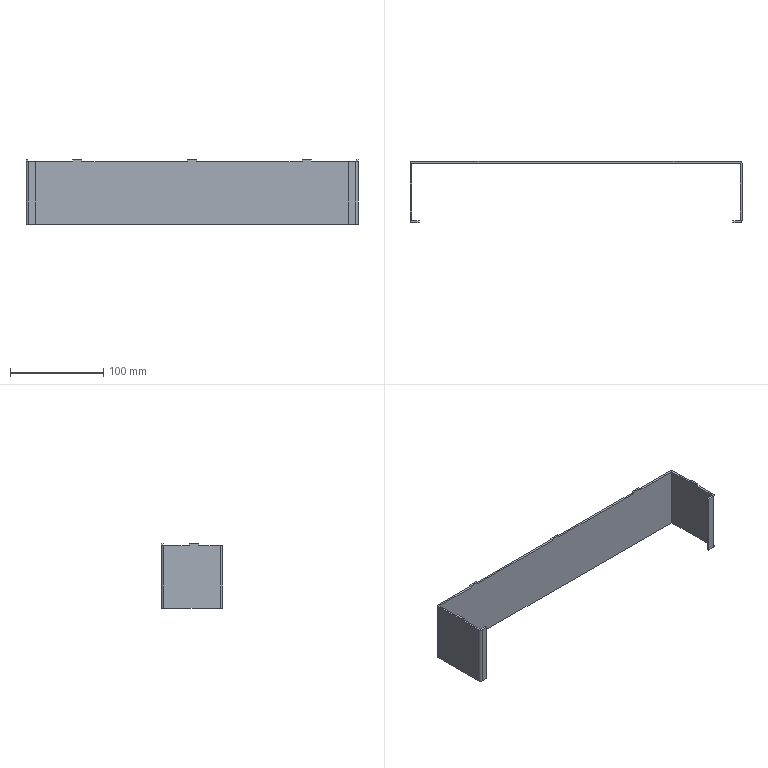Part | STEP file | xzz-005 | 1 solid | 42 faces | box 356 x 66 x 69 mm | volume 66855 mm3 | plane 34 | cylinder 8 | commonest cylinder face diameters 1 x4 5 x4
STEP:
#1=CARTESIAN_POINT('',(198.5,6.,67.));
#2=VERTEX_POINT('',#1);
#3=CARTESIAN_POINT('',(198.5,6.,0.));
#4=VERTEX_POINT('',#3);
#5=CARTESIAN_POINT('',(198.5,6.,67.));
#6=DIRECTION('',(0.,0.,-1.));
#7=VECTOR('',#6,1000.);
#8=LINE('',#5,#7);
#9=EDGE_CURVE('',#2,#4,#8,.T.);
#10=ORIENTED_EDGE('',*,*,#9,.F.);
#11=CARTESIAN_POINT('',(151.,6.,67.));
#12=VERTEX_POINT('',#11);
#13=CARTESIAN_POINT('',(-155.,6.,67.));
#14=DIRECTION('',(1.,0.,0.));
#15=VECTOR('',#14,1000.);
#16=LINE('',#13,#15);
#17=EDGE_CURVE('',#12,#2,#16,.T.);
#18=ORIENTED_EDGE('',*,*,#17,.F.);
#19=CARTESIAN_POINT('',(151.,6.,69.));
#20=VERTEX_POINT('',#19);
#21=CARTESIAN_POINT('',(151.,6.,67.));
#22=DIRECTION('',(0.,0.,-1.));
#23=VECTOR('',#22,1000.);
#24=LINE('',#21,#23);
#25=EDGE_CURVE('',#20,#12,#24,.T.);
#26=ORIENTED_EDGE('',*,*,#25,.F.);
#27=CARTESIAN_POINT('',(141.,6.,69.));
#28=VERTEX_POINT('',#27);
#29=CARTESIAN_POINT('',(-155.,6.,69.));
#30=DIRECTION('',(1.,0.,0.));
#31=VECTOR('',#30,1000.);
#32=LINE('',#29,#31);
#33=EDGE_CURVE('',#28,#20,#32,.T.);
#34=ORIENTED_EDGE('',*,*,#33,.F.);
#35=CARTESIAN_POINT('',(141.,6.,67.));
#36=VERTEX_POINT('',#35);
#37=CARTESIAN_POINT('',(141.,6.,67.));
#38=DIRECTION('',(0.,0.,1.));
#39=VECTOR('',#38,1000.);
#40=LINE('',#37,#39);
#41=EDGE_CURVE('',#36,#28,#40,.T.);
#42=ORIENTED_EDGE('',*,*,#41,.F.);
#43=CARTESIAN_POINT('',(28.,6.,67.));
#44=VERTEX_POINT('',#43);
#45=CARTESIAN_POINT('',(-155.,6.,67.));
#46=DIRECTION('',(1.,0.,0.));
#47=VECTOR('',#46,1000.);
#48=LINE('',#45,#47);
#49=EDGE_CURVE('',#44,#36,#48,.T.);
#50=ORIENTED_EDGE('',*,*,#49,.F.);
#51=CARTESIAN_POINT('',(28.,6.,69.));
#52=VERTEX_POINT('',#51);
#53=CARTESIAN_POINT('',(28.,6.,67.));
#54=DIRECTION('',(0.,0.,-1.));
#55=VECTOR('',#54,1000.);
#56=LINE('',#53,#55);
#57=EDGE_CURVE('',#52,#44,#56,.T.);
#58=ORIENTED_EDGE('',*,*,#57,.F.);
#59=CARTESIAN_POINT('',(18.,6.,69.));
#60=VERTEX_POINT('',#59);
#61=CARTESIAN_POINT('',(-155.,6.,69.));
#62=DIRECTION('',(1.,0.,0.));
#63=VECTOR('',#62,1000.);
#64=LINE('',#61,#63);
#65=EDGE_CURVE('',#60,#52,#64,.T.);
#66=ORIENTED_EDGE('',*,*,#65,.F.);
#67=CARTESIAN_POINT('',(18.,6.,67.));
#68=VERTEX_POINT('',#67);
#69=CARTESIAN_POINT('',(18.,6.,67.));
#70=DIRECTION('',(0.,0.,1.));
#71=VECTOR('',#70,1000.);
#72=LINE('',#69,#71);
#73=EDGE_CURVE('',#68,#60,#72,.T.);
#74=ORIENTED_EDGE('',*,*,#73,.F.);
#75=CARTESIAN_POINT('',(-95.,6.,67.));
#76=VERTEX_POINT('',#75);
#77=CARTESIAN_POINT('',(-155.,6.,67.));
#78=DIRECTION('',(1.,0.,0.));
#79=VECTOR('',#78,1000.);
#80=LINE('',#77,#79);
#81=EDGE_CURVE('',#76,#68,#80,.T.);
#82=ORIENTED_EDGE('',*,*,#81,.F.);
#83=CARTESIAN_POINT('',(-95.,6.,69.));
#84=VERTEX_POINT('',#83);
#85=CARTESIAN_POINT('',(-95.,6.,67.));
#86=DIRECTION('',(0.,0.,-1.));
#87=VECTOR('',#86,1000.);
#88=LINE('',#85,#87);
#89=EDGE_CURVE('',#84,#76,#88,.T.);
#90=ORIENTED_EDGE('',*,*,#89,.F.);
#91=CARTESIAN_POINT('',(-105.,6.,69.));
#92=VERTEX_POINT('',#91);
#93=CARTESIAN_POINT('',(-155.,6.,69.));
#94=DIRECTION('',(1.,0.,0.));
#95=VECTOR('',#94,1000.);
#96=LINE('',#93,#95);
#97=EDGE_CURVE('',#92,#84,#96,.T.);
#98=ORIENTED_EDGE('',*,*,#97,.F.);
#99=CARTESIAN_POINT('',(-105.,6.,67.));
#100=VERTEX_POINT('',#99);
#101=CARTESIAN_POINT('',(-105.,6.,67.));
#102=DIRECTION('',(0.,0.,1.));
#103=VECTOR('',#102,1000.);
#104=LINE('',#101,#103);
#105=EDGE_CURVE('',#100,#92,#104,.T.);
#106=ORIENTED_EDGE('',*,*,#105,.F.);
#107=CARTESIAN_POINT('',(-152.5,6.,67.));
#108=VERTEX_POINT('',#107);
#109=CARTESIAN_POINT('',(-155.,6.,67.));
#110=DIRECTION('',(1.,0.,0.));
#111=VECTOR('',#110,1000.);
#112=LINE('',#109,#111);
#113=EDGE_CURVE('',#108,#100,#112,.T.);
#114=ORIENTED_EDGE('',*,*,#113,.F.);
#115=CARTESIAN_POINT('',(-152.5,6.,0.));
#116=VERTEX_POINT('',#115);
#117=CARTESIAN_POINT('',(-152.5,6.,67.));
#118=DIRECTION('',(0.,0.,1.));
#119=VECTOR('',#118,1000.);
#120=LINE('',#117,#119);
#121=EDGE_CURVE('',#116,#108,#120,.T.);
#122=ORIENTED_EDGE('',*,*,#121,.F.);
#123=CARTESIAN_POINT('',(-155.,6.,0.));
#124=DIRECTION('',(-1.,0.,0.));
#125=VECTOR('',#124,1000.);
#126=LINE('',#123,#125);
#127=EDGE_CURVE('',#4,#116,#126,.T.);
#128=ORIENTED_EDGE('',*,*,#127,.F.);
#129=EDGE_LOOP('',(#10,#18,#26,#34,#42,#50,#58,#66,#74,#82,#90,#98,#106,#114,#122,#128));
#130=FACE_OUTER_BOUND('',#129,.T.);
#131=CARTESIAN_POINT('',(-155.,6.,67.));
#132=DIRECTION('',(0.,1.,0.));
#133=DIRECTION('',(0.,0.,1.));
#134=AXIS2_PLACEMENT_3D('',#131,#132,#133);
#135=PLANE('',#134);
#136=ADVANCED_FACE('',(#130),#135,.F.);
#137=ORIENTED_EDGE('',*,*,#127,.T.);
#138=CARTESIAN_POINT('',(-153.,5.5,0.));
#139=VERTEX_POINT('',#138);
#140=CARTESIAN_POINT('',(-152.5,5.5,0.));
#141=DIRECTION('',(0.,0.,1.));
#142=DIRECTION('',(-1.,0.,0.));
#143=AXIS2_PLACEMENT_3D('',#140,#141,#142);
#144=CIRCLE('',#143,0.5);
#145=EDGE_CURVE('',#116,#139,#144,.T.);
#146=ORIENTED_EDGE('',*,*,#145,.T.);
#147=CARTESIAN_POINT('',(-153.,-55.5,0.));
#148=VERTEX_POINT('',#147);
#149=CARTESIAN_POINT('',(-153.,8.,0.));
#150=DIRECTION('',(0.,-1.,0.));
#151=VECTOR('',#150,1000.);
#152=LINE('',#149,#151);
#153=EDGE_CURVE('',#139,#148,#152,.T.);
#154=ORIENTED_EDGE('',*,*,#153,.T.);
#155=CARTESIAN_POINT('',(-152.5,-56.,0.));
#156=VERTEX_POINT('',#155);
#157=CARTESIAN_POINT('',(-152.5,-55.5,0.));
#158=DIRECTION('',(0.,0.,1.));
#159=DIRECTION('',(-1.,0.,0.));
#160=AXIS2_PLACEMENT_3D('',#157,#158,#159);
#161=CIRCLE('',#160,0.5);
#162=EDGE_CURVE('',#148,#156,#161,.T.);
#163=ORIENTED_EDGE('',*,*,#162,.T.);
#164=CARTESIAN_POINT('',(-145.,-56.,0.));
#165=VERTEX_POINT('',#164);
#166=CARTESIAN_POINT('',(-155.,-56.,0.));
#167=DIRECTION('',(1.,0.,0.));
#168=VECTOR('',#167,1000.);
#169=LINE('',#166,#168);
#170=EDGE_CURVE('',#156,#165,#169,.T.);
#171=ORIENTED_EDGE('',*,*,#170,.T.);
#172=CARTESIAN_POINT('',(-145.,-58.,0.));
#173=VERTEX_POINT('',#172);
#174=CARTESIAN_POINT('',(-145.,-55.5,0.));
#175=DIRECTION('',(0.,-1.,0.));
#176=VECTOR('',#175,1000.);
#177=LINE('',#174,#176);
#178=EDGE_CURVE('',#165,#173,#177,.T.);
#179=ORIENTED_EDGE('',*,*,#178,.T.);
#180=CARTESIAN_POINT('',(-152.5,-58.,0.));
#181=VERTEX_POINT('',#180);
#182=CARTESIAN_POINT('',(-153.,-58.,0.));
#183=DIRECTION('',(-1.,0.,0.));
#184=VECTOR('',#183,1000.);
#185=LINE('',#182,#184);
#186=EDGE_CURVE('',#173,#181,#185,.T.);
#187=ORIENTED_EDGE('',*,*,#186,.T.);
#188=CARTESIAN_POINT('',(-155.,-55.5,0.));
#189=VERTEX_POINT('',#188);
#190=CARTESIAN_POINT('',(-152.5,-55.5,0.));
#191=DIRECTION('',(0.,0.,-1.));
#192=DIRECTION('',(-1.,0.,0.));
#193=AXIS2_PLACEMENT_3D('',#190,#191,#192);
#194=CIRCLE('',#193,2.5);
#195=EDGE_CURVE('',#181,#189,#194,.T.);
#196=ORIENTED_EDGE('',*,*,#195,.T.);
#197=CARTESIAN_POINT('',(-155.,5.5,0.));
#198=VERTEX_POINT('',#197);
#199=CARTESIAN_POINT('',(-155.,6.,0.));
#200=DIRECTION('',(0.,1.,0.));
#201=VECTOR('',#200,1000.);
#202=LINE('',#199,#201);
#203=EDGE_CURVE('',#189,#198,#202,.T.);
#204=ORIENTED_EDGE('',*,*,#203,.T.);
#205=CARTESIAN_POINT('',(-152.5,8.,0.));
#206=VERTEX_POINT('',#205);
#207=CARTESIAN_POINT('',(-152.5,5.5,0.));
#208=DIRECTION('',(0.,0.,-1.));
#209=DIRECTION('',(-1.,0.,0.));
#210=AXIS2_PLACEMENT_3D('',#207,#208,#209);
#211=CIRCLE('',#210,2.5);
#212=EDGE_CURVE('',#198,#206,#211,.T.);
#213=ORIENTED_EDGE('',*,*,#212,.T.);
#214=CARTESIAN_POINT('',(198.5,8.,0.));
#215=VERTEX_POINT('',#214);
#216=CARTESIAN_POINT('',(199.,8.,0.));
#217=DIRECTION('',(1.,0.,0.));
#218=VECTOR('',#217,1000.);
#219=LINE('',#216,#218);
#220=EDGE_CURVE('',#206,#215,#219,.T.);
#221=ORIENTED_EDGE('',*,*,#220,.T.);
#222=CARTESIAN_POINT('',(201.,5.5,0.));
#223=VERTEX_POINT('',#222);
#224=CARTESIAN_POINT('',(198.5,5.5,0.));
#225=DIRECTION('',(0.,0.,-1.));
#226=DIRECTION('',(-1.,0.,0.));
#227=AXIS2_PLACEMENT_3D('',#224,#225,#226);
#228=CIRCLE('',#227,2.5);
#229=EDGE_CURVE('',#215,#223,#228,.T.);
#230=ORIENTED_EDGE('',*,*,#229,.T.);
#231=CARTESIAN_POINT('',(201.,-55.5,0.));
#232=VERTEX_POINT('',#231);
#233=CARTESIAN_POINT('',(201.,-56.,0.));
#234=DIRECTION('',(0.,-1.,0.));
#235=VECTOR('',#234,1000.);
#236=LINE('',#233,#235);
#237=EDGE_CURVE('',#223,#232,#236,.T.);
#238=ORIENTED_EDGE('',*,*,#237,.T.);
#239=CARTESIAN_POINT('',(198.5,-58.,0.));
#240=VERTEX_POINT('',#239);
#241=CARTESIAN_POINT('',(198.5,-55.5,0.));
#242=DIRECTION('',(0.,0.,-1.));
#243=DIRECTION('',(-1.,0.,0.));
#244=AXIS2_PLACEMENT_3D('',#241,#242,#243);
#245=CIRCLE('',#244,2.5);
#246=EDGE_CURVE('',#232,#240,#245,.T.);
#247=ORIENTED_EDGE('',*,*,#246,.T.);
#248=CARTESIAN_POINT('',(191.,-58.,0.));
#249=VERTEX_POINT('',#248);
#250=CARTESIAN_POINT('',(198.5,-58.,0.));
#251=DIRECTION('',(1.,0.,0.));
#252=VECTOR('',#251,1000.);
#253=LINE('',#250,#252);
#254=EDGE_CURVE('',#249,#240,#253,.T.);
#255=ORIENTED_EDGE('',*,*,#254,.F.);
#256=CARTESIAN_POINT('',(191.,-56.,0.));
#257=VERTEX_POINT('',#256);
#258=CARTESIAN_POINT('',(191.,-55.5,0.));
#259=DIRECTION('',(0.,-1.,0.));
#260=VECTOR('',#259,1000.);
#261=LINE('',#258,#260);
#262=EDGE_CURVE('',#257,#249,#261,.T.);
#263=ORIENTED_EDGE('',*,*,#262,.F.);
#264=CARTESIAN_POINT('',(198.5,-56.,0.));
#265=VERTEX_POINT('',#264);
#266=CARTESIAN_POINT('',(201.,-56.,0.));
#267=DIRECTION('',(1.,0.,0.));
#268=VECTOR('',#267,1000.);
#269=LINE('',#266,#268);
#270=EDGE_CURVE('',#257,#265,#269,.T.);
#271=ORIENTED_EDGE('',*,*,#270,.T.);
#272=CARTESIAN_POINT('',(199.,-55.5,0.));
#273=VERTEX_POINT('',#272);
#274=CARTESIAN_POINT('',(198.5,-55.5,0.));
#275=DIRECTION('',(0.,0.,1.));
#276=DIRECTION('',(-1.,0.,0.));
#277=AXIS2_PLACEMENT_3D('',#274,#275,#276);
#278=CIRCLE('',#277,0.5);
#279=EDGE_CURVE('',#265,#273,#278,.T.);
#280=ORIENTED_EDGE('',*,*,#279,.T.);
#281=CARTESIAN_POINT('',(199.,5.5,0.));
#282=VERTEX_POINT('',#281);
#283=CARTESIAN_POINT('',(199.,8.,0.));
#284=DIRECTION('',(0.,1.,0.));
#285=VECTOR('',#284,1000.);
#286=LINE('',#283,#285);
#287=EDGE_CURVE('',#273,#282,#286,.T.);
#288=ORIENTED_EDGE('',*,*,#287,.T.);
#289=CARTESIAN_POINT('',(198.5,5.5,0.));
#290=DIRECTION('',(0.,0.,1.));
#291=DIRECTION('',(-1.,0.,0.));
#292=AXIS2_PLACEMENT_3D('',#289,#290,#291);
#293=CIRCLE('',#292,0.5);
#294=EDGE_CURVE('',#282,#4,#293,.T.);
#295=ORIENTED_EDGE('',*,*,#294,.T.);
#296=EDGE_LOOP('',(#137,#146,#154,#163,#171,#179,#187,#196,#204,#213,#221,#230,#238,#247,#255,#263,#271,#280,#288,#295));
#297=FACE_OUTER_BOUND('',#296,.T.);
#298=CARTESIAN_POINT('',(199.,5.5,0.));
#299=DIRECTION('',(0.,0.,-1.));
#300=DIRECTION('',(-1.,0.,0.));
#301=AXIS2_PLACEMENT_3D('',#298,#299,#300);
#302=PLANE('',#301);
#303=ADVANCED_FACE('',(#297),#302,.T.);
#304=CARTESIAN_POINT('',(199.,5.5,67.));
#305=VERTEX_POINT('',#304);
#306=CARTESIAN_POINT('',(199.,5.5,67.));
#307=DIRECTION('',(0.,0.,-1.));
#308=VECTOR('',#307,1000.);
#309=LINE('',#306,#308);
#310=EDGE_CURVE('',#305,#282,#309,.T.);
#311=ORIENTED_EDGE('',*,*,#310,.F.);
#312=CARTESIAN_POINT('',(198.5,5.5,67.));
#313=DIRECTION('',(0.,0.,-1.));
#314=DIRECTION('',(-1.,0.,0.));
#315=AXIS2_PLACEMENT_3D('',#312,#313,#314);
#316=CIRCLE('',#315,0.5);
#317=EDGE_CURVE('',#2,#305,#316,.T.);
#318=ORIENTED_EDGE('',*,*,#317,.F.);
#319=ORIENTED_EDGE('',*,*,#9,.T.);
#320=ORIENTED_EDGE('',*,*,#294,.F.);
#321=EDGE_LOOP('',(#311,#318,#319,#320));
#322=FACE_OUTER_BOUND('',#321,.T.);
#323=CARTESIAN_POINT('',(198.5,5.5,67.));
#324=DIRECTION('',(0.,0.,-1.));
#325=DIRECTION('',(-1.,0.,0.));
#326=AXIS2_PLACEMENT_3D('',#323,#324,#325);
#327=CYLINDRICAL_SURFACE('',#326,0.5);
#328=ADVANCED_FACE('',(#322),#327,.F.);
#329=ORIENTED_EDGE('',*,*,#17,.T.);
#330=ORIENTED_EDGE('',*,*,#317,.T.);
#331=CARTESIAN_POINT('',(199.,-22.,67.));
#332=VERTEX_POINT('',#331);
#333=CARTESIAN_POINT('',(199.,8.,67.));
#334=DIRECTION('',(0.,-1.,0.));
#335=VECTOR('',#334,1000.);
#336=LINE('',#333,#335);
#337=EDGE_CURVE('',#305,#332,#336,.T.);
#338=ORIENTED_EDGE('',*,*,#337,.T.);
#339=CARTESIAN_POINT('',(201.,-22.,67.));
#340=VERTEX_POINT('',#339);
#341=CARTESIAN_POINT('',(199.,-22.,67.));
#342=DIRECTION('',(1.,0.,0.));
#343=VECTOR('',#342,1000.);
#344=LINE('',#341,#343);
#345=EDGE_CURVE('',#332,#340,#344,.T.);
#346=ORIENTED_EDGE('',*,*,#345,.T.);
#347=CARTESIAN_POINT('',(201.,5.5,67.));
#348=VERTEX_POINT('',#347);
#349=CARTESIAN_POINT('',(201.,6.,67.));
#350=DIRECTION('',(0.,1.,0.));
#351=VECTOR('',#350,1000.);
#352=LINE('',#349,#351);
#353=EDGE_CURVE('',#340,#348,#352,.T.);
#354=ORIENTED_EDGE('',*,*,#353,.T.);
#355=CARTESIAN_POINT('',(198.5,8.,67.));
#356=VERTEX_POINT('',#355);
#357=CARTESIAN_POINT('',(198.5,5.5,67.));
#358=DIRECTION('',(0.,0.,1.));
#359=DIRECTION('',(-1.,0.,0.));
#360=AXIS2_PLACEMENT_3D('',#357,#358,#359);
#361=CIRCLE('',#360,2.5);
#362=EDGE_CURVE('',#348,#356,#361,.T.);
#363=ORIENTED_EDGE('',*,*,#362,.T.);
#364=CARTESIAN_POINT('',(151.,8.,67.));
#365=VERTEX_POINT('',#364);
#366=CARTESIAN_POINT('',(-153.,8.,67.));
#367=DIRECTION('',(-1.,0.,0.));
#368=VECTOR('',#367,1000.);
#369=LINE('',#366,#368);
#370=EDGE_CURVE('',#356,#365,#369,.T.);
#371=ORIENTED_EDGE('',*,*,#370,.T.);
#372=CARTESIAN_POINT('',(151.,5.5,67.));
#373=DIRECTION('',(0.,-1.,0.));
#374=VECTOR('',#373,1000.);
#375=LINE('',#372,#374);
#376=EDGE_CURVE('',#365,#12,#375,.T.);
#377=ORIENTED_EDGE('',*,*,#376,.T.);
#378=EDGE_LOOP('',(#329,#330,#338,#346,#354,#363,#371,#377));
#379=FACE_OUTER_BOUND('',#378,.T.);
#380=CARTESIAN_POINT('',(-153.,5.5,67.));
#381=DIRECTION('',(0.,0.,1.));
#382=DIRECTION('',(1.,0.,0.));
#383=AXIS2_PLACEMENT_3D('',#380,#381,#382);
#384=PLANE('',#383);
#385=ADVANCED_FACE('',(#379),#384,.T.);
#386=CARTESIAN_POINT('',(151.,8.,69.));
#387=VERTEX_POINT('',#386);
#388=CARTESIAN_POINT('',(151.,8.,69.));
#389=DIRECTION('',(0.,0.,-1.));
#390=VECTOR('',#389,1000.);
#391=LINE('',#388,#390);
#392=EDGE_CURVE('',#387,#365,#391,.T.);
#393=ORIENTED_EDGE('',*,*,#392,.F.);
#394=CARTESIAN_POINT('',(151.,8.,69.));
#395=DIRECTION('',(0.,1.,0.));
#396=VECTOR('',#395,1000.);
#397=LINE('',#394,#396);
#398=EDGE_CURVE('',#20,#387,#397,.T.);
#399=ORIENTED_EDGE('',*,*,#398,.F.);
#400=ORIENTED_EDGE('',*,*,#25,.T.);
#401=ORIENTED_EDGE('',*,*,#376,.F.);
#402=EDGE_LOOP('',(#393,#399,#400,#401));
#403=FACE_OUTER_BOUND('',#402,.T.);
#404=CARTESIAN_POINT('',(151.,8.,69.));
#405=DIRECTION('',(-1.,0.,0.));
#406=DIRECTION('',(0.,0.,1.));
#407=AXIS2_PLACEMENT_3D('',#404,#405,#406);
#408=PLANE('',#407);
#409=ADVANCED_FACE('',(#403),#408,.F.);
#410=ORIENTED_EDGE('',*,*,#398,.T.);
#411=CARTESIAN_POINT('',(141.,8.,69.));
#412=VERTEX_POINT('',#411);
#413=CARTESIAN_POINT('',(0.,8.,69.));
#414=DIRECTION('',(-1.,0.,0.));
#415=VECTOR('',#414,1000.);
#416=LINE('',#413,#415);
#417=EDGE_CURVE('',#387,#412,#416,.T.);
#418=ORIENTED_EDGE('',*,*,#417,.T.);
#419=CARTESIAN_POINT('',(141.,0.,69.));
#420=DIRECTION('',(0.,-1.,0.));
#421=VECTOR('',#420,1000.);
#422=LINE('',#419,#421);
#423=EDGE_CURVE('',#412,#28,#422,.T.);
#424=ORIENTED_EDGE('',*,*,#423,.T.);
#425=ORIENTED_EDGE('',*,*,#33,.T.);
#426=EDGE_LOOP('',(#410,#418,#424,#425));
#427=FACE_OUTER_BOUND('',#426,.T.);
#428=CARTESIAN_POINT('',(0.,0.,69.));
#429=DIRECTION('',(0.,0.,1.));
#430=DIRECTION('',(1.,0.,0.));
#431=AXIS2_PLACEMENT_3D('',#428,#429,#430);
#432=PLANE('',#431);
#433=ADVANCED_FACE('',(#427),#432,.T.);
#434=ORIENTED_EDGE('',*,*,#41,.T.);
#435=ORIENTED_EDGE('',*,*,#423,.F.);
#436=CARTESIAN_POINT('',(141.,8.,67.));
#437=VERTEX_POINT('',#436);
#438=CARTESIAN_POINT('',(141.,8.,69.));
#439=DIRECTION('',(0.,0.,1.));
#440=VECTOR('',#439,1000.);
#441=LINE('',#438,#440);
#442=EDGE_CURVE('',#437,#412,#441,.T.);
#443=ORIENTED_EDGE('',*,*,#442,.F.);
#444=CARTESIAN_POINT('',(141.,8.,67.));
#445=DIRECTION('',(0.,1.,0.));
#446=VECTOR('',#445,1000.);
#447=LINE('',#444,#446);
#448=EDGE_CURVE('',#36,#437,#447,.T.);
#449=ORIENTED_EDGE('',*,*,#448,.F.);
#450=EDGE_LOOP('',(#434,#435,#443,#449));
#451=FACE_OUTER_BOUND('',#450,.T.);
#452=CARTESIAN_POINT('',(141.,8.,69.));
#453=DIRECTION('',(1.,0.,0.));
#454=DIRECTION('',(0.,0.,-1.));
#455=AXIS2_PLACEMENT_3D('',#452,#453,#454);
#456=PLANE('',#455);
#457=ADVANCED_FACE('',(#451),#456,.F.);
#458=ORIENTED_EDGE('',*,*,#49,.T.);
#459=ORIENTED_EDGE('',*,*,#448,.T.);
#460=CARTESIAN_POINT('',(28.,8.,67.));
#461=VERTEX_POINT('',#460);
#462=CARTESIAN_POINT('',(-153.,8.,67.));
#463=DIRECTION('',(-1.,0.,0.));
#464=VECTOR('',#463,1000.);
#465=LINE('',#462,#464);
#466=EDGE_CURVE('',#437,#461,#465,.T.);
#467=ORIENTED_EDGE('',*,*,#466,.T.);
#468=CARTESIAN_POINT('',(28.,5.5,67.));
#469=DIRECTION('',(0.,-1.,0.));
#470=VECTOR('',#469,1000.);
#471=LINE('',#468,#470);
#472=EDGE_CURVE('',#461,#44,#471,.T.);
#473=ORIENTED_EDGE('',*,*,#472,.T.);
#474=EDGE_LOOP('',(#458,#459,#467,#473));
#475=FACE_OUTER_BOUND('',#474,.T.);
#476=CARTESIAN_POINT('',(-153.,5.5,67.));
#477=DIRECTION('',(0.,0.,1.));
#478=DIRECTION('',(1.,0.,0.));
#479=AXIS2_PLACEMENT_3D('',#476,#477,#478);
#480=PLANE('',#479);
#481=ADVANCED_FACE('',(#475),#480,.T.);
#482=CARTESIAN_POINT('',(28.,8.,69.));
#483=VERTEX_POINT('',#482);
#484=CARTESIAN_POINT('',(28.,8.,69.));
#485=DIRECTION('',(0.,0.,-1.));
#486=VECTOR('',#485,1000.);
#487=LINE('',#484,#486);
#488=EDGE_CURVE('',#483,#461,#487,.T.);
#489=ORIENTED_EDGE('',*,*,#488,.F.);
#490=CARTESIAN_POINT('',(28.,8.,69.));
#491=DIRECTION('',(0.,1.,0.));
#492=VECTOR('',#491,1000.);
#493=LINE('',#490,#492);
#494=EDGE_CURVE('',#52,#483,#493,.T.);
#495=ORIENTED_EDGE('',*,*,#494,.F.);
#496=ORIENTED_EDGE('',*,*,#57,.T.);
#497=ORIENTED_EDGE('',*,*,#472,.F.);
#498=EDGE_LOOP('',(#489,#495,#496,#497));
#499=FACE_OUTER_BOUND('',#498,.T.);
#500=CARTESIAN_POINT('',(28.,8.,69.));
#501=DIRECTION('',(-1.,0.,0.));
#502=DIRECTION('',(0.,0.,1.));
#503=AXIS2_PLACEMENT_3D('',#500,#501,#502);
#504=PLANE('',#503);
#505=ADVANCED_FACE('',(#499),#504,.F.);
#506=ORIENTED_EDGE('',*,*,#494,.T.);
#507=CARTESIAN_POINT('',(18.,8.,69.));
#508=VERTEX_POINT('',#507);
#509=CARTESIAN_POINT('',(0.,8.,69.));
#510=DIRECTION('',(-1.,0.,0.));
#511=VECTOR('',#510,1000.);
#512=LINE('',#509,#511);
#513=EDGE_CURVE('',#483,#508,#512,.T.);
#514=ORIENTED_EDGE('',*,*,#513,.T.);
#515=CARTESIAN_POINT('',(18.,0.,69.));
#516=DIRECTION('',(0.,-1.,0.));
#517=VECTOR('',#516,1000.);
#518=LINE('',#515,#517);
#519=EDGE_CURVE('',#508,#60,#518,.T.);
#520=ORIENTED_EDGE('',*,*,#519,.T.);
#521=ORIENTED_EDGE('',*,*,#65,.T.);
#522=EDGE_LOOP('',(#506,#514,#520,#521));
#523=FACE_OUTER_BOUND('',#522,.T.);
#524=CARTESIAN_POINT('',(0.,0.,69.));
#525=DIRECTION('',(0.,0.,1.));
#526=DIRECTION('',(1.,0.,0.));
#527=AXIS2_PLACEMENT_3D('',#524,#525,#526);
#528=PLANE('',#527);
#529=ADVANCED_FACE('',(#523),#528,.T.);
#530=ORIENTED_EDGE('',*,*,#73,.T.);
#531=ORIENTED_EDGE('',*,*,#519,.F.);
#532=CARTESIAN_POINT('',(18.,8.,67.));
#533=VERTEX_POINT('',#532);
#534=CARTESIAN_POINT('',(18.,8.,69.));
#535=DIRECTION('',(0.,0.,1.));
#536=VECTOR('',#535,1000.);
#537=LINE('',#534,#536);
#538=EDGE_CURVE('',#533,#508,#537,.T.);
#539=ORIENTED_EDGE('',*,*,#538,.F.);
#540=CARTESIAN_POINT('',(18.,8.,67.));
#541=DIRECTION('',(0.,1.,0.));
#542=VECTOR('',#541,1000.);
#543=LINE('',#540,#542);
#544=EDGE_CURVE('',#68,#533,#543,.T.);
#545=ORIENTED_EDGE('',*,*,#544,.F.);
#546=EDGE_LOOP('',(#530,#531,#539,#545));
#547=FACE_OUTER_BOUND('',#546,.T.);
#548=CARTESIAN_POINT('',(18.,8.,69.));
#549=DIRECTION('',(1.,0.,0.));
#550=DIRECTION('',(0.,0.,-1.));
#551=AXIS2_PLACEMENT_3D('',#548,#549,#550);
#552=PLANE('',#551);
#553=ADVANCED_FACE('',(#547),#552,.F.);
#554=CARTESIAN_POINT('',(-95.,8.,67.));
#555=VERTEX_POINT('',#554);
#556=CARTESIAN_POINT('',(-153.,8.,67.));
#557=DIRECTION('',(-1.,0.,0.));
#558=VECTOR('',#557,1000.);
#559=LINE('',#556,#558);
#560=EDGE_CURVE('',#533,#555,#559,.T.);
#561=ORIENTED_EDGE('',*,*,#560,.T.);
#562=CARTESIAN_POINT('',(-95.,5.5,67.));
#563=DIRECTION('',(0.,-1.,0.));
#564=VECTOR('',#563,1000.);
#565=LINE('',#562,#564);
#566=EDGE_CURVE('',#555,#76,#565,.T.);
#567=ORIENTED_EDGE('',*,*,#566,.T.);
#568=ORIENTED_EDGE('',*,*,#81,.T.);
#569=ORIENTED_EDGE('',*,*,#544,.T.);
#570=EDGE_LOOP('',(#561,#567,#568,#569));
#571=FACE_OUTER_BOUND('',#570,.T.);
#572=CARTESIAN_POINT('',(-153.,5.5,67.));
#573=DIRECTION('',(0.,0.,1.));
#574=DIRECTION('',(1.,0.,0.));
#575=AXIS2_PLACEMENT_3D('',#572,#573,#574);
#576=PLANE('',#575);
#577=ADVANCED_FACE('',(#571),#576,.T.);
#578=CARTESIAN_POINT('',(-95.,8.,69.));
#579=VERTEX_POINT('',#578);
#580=CARTESIAN_POINT('',(-95.,8.,69.));
#581=DIRECTION('',(0.,0.,-1.));
#582=VECTOR('',#581,1000.);
#583=LINE('',#580,#582);
#584=EDGE_CURVE('',#579,#555,#583,.T.);
#585=ORIENTED_EDGE('',*,*,#584,.F.);
#586=CARTESIAN_POINT('',(-95.,8.,69.));
#587=DIRECTION('',(0.,1.,0.));
#588=VECTOR('',#587,1000.);
#589=LINE('',#586,#588);
#590=EDGE_CURVE('',#84,#579,#589,.T.);
#591=ORIENTED_EDGE('',*,*,#590,.F.);
#592=ORIENTED_EDGE('',*,*,#89,.T.);
#593=ORIENTED_EDGE('',*,*,#566,.F.);
#594=EDGE_LOOP('',(#585,#591,#592,#593));
#595=FACE_OUTER_BOUND('',#594,.T.);
#596=CARTESIAN_POINT('',(-95.,8.,69.));
#597=DIRECTION('',(-1.,0.,0.));
#598=DIRECTION('',(0.,0.,1.));
#599=AXIS2_PLACEMENT_3D('',#596,#597,#598);
#600=PLANE('',#599);
#601=ADVANCED_FACE('',(#595),#600,.F.);
#602=ORIENTED_EDGE('',*,*,#590,.T.);
#603=CARTESIAN_POINT('',(-105.,8.,69.));
#604=VERTEX_POINT('',#603);
#605=CARTESIAN_POINT('',(0.,8.,69.));
#606=DIRECTION('',(-1.,0.,0.));
#607=VECTOR('',#606,1000.);
#608=LINE('',#605,#607);
#609=EDGE_CURVE('',#579,#604,#608,.T.);
#610=ORIENTED_EDGE('',*,*,#609,.T.);
#611=CARTESIAN_POINT('',(-105.,0.,69.));
#612=DIRECTION('',(0.,-1.,0.));
#613=VECTOR('',#612,1000.);
#614=LINE('',#611,#613);
#615=EDGE_CURVE('',#604,#92,#614,.T.);
#616=ORIENTED_EDGE('',*,*,#615,.T.);
#617=ORIENTED_EDGE('',*,*,#97,.T.);
#618=EDGE_LOOP('',(#602,#610,#616,#617));
#619=FACE_OUTER_BOUND('',#618,.T.);
#620=CARTESIAN_POINT('',(0.,0.,69.));
#621=DIRECTION('',(0.,0.,1.));
#622=DIRECTION('',(1.,0.,0.));
#623=AXIS2_PLACEMENT_3D('',#620,#621,#622);
#624=PLANE('',#623);
#625=ADVANCED_FACE('',(#619),#624,.T.);
#626=ORIENTED_EDGE('',*,*,#105,.T.);
#627=ORIENTED_EDGE('',*,*,#615,.F.);
#628=CARTESIAN_POINT('',(-105.,8.,67.));
#629=VERTEX_POINT('',#628);
#630=CARTESIAN_POINT('',(-105.,8.,69.));
#631=DIRECTION('',(0.,0.,1.));
#632=VECTOR('',#631,1000.);
#633=LINE('',#630,#632);
#634=EDGE_CURVE('',#629,#604,#633,.T.);
#635=ORIENTED_EDGE('',*,*,#634,.F.);
#636=CARTESIAN_POINT('',(-105.,8.,67.));
#637=DIRECTION('',(0.,1.,0.));
#638=VECTOR('',#637,1000.);
#639=LINE('',#636,#638);
#640=EDGE_CURVE('',#100,#629,#639,.T.);
#641=ORIENTED_EDGE('',*,*,#640,.F.);
#642=EDGE_LOOP('',(#626,#627,#635,#641));
#643=FACE_OUTER_BOUND('',#642,.T.);
#644=CARTESIAN_POINT('',(-105.,8.,69.));
#645=DIRECTION('',(1.,0.,0.));
#646=DIRECTION('',(0.,0.,-1.));
#647=AXIS2_PLACEMENT_3D('',#644,#645,#646);
#648=PLANE('',#647);
#649=ADVANCED_FACE('',(#643),#648,.F.);
#650=CARTESIAN_POINT('',(-152.5,8.,67.));
#651=VERTEX_POINT('',#650);
#652=CARTESIAN_POINT('',(-153.,8.,67.));
#653=DIRECTION('',(-1.,0.,0.));
#654=VECTOR('',#653,1000.);
#655=LINE('',#652,#654);
#656=EDGE_CURVE('',#629,#651,#655,.T.);
#657=ORIENTED_EDGE('',*,*,#656,.T.);
#658=CARTESIAN_POINT('',(-155.,5.5,67.));
#659=VERTEX_POINT('',#658);
#660=CARTESIAN_POINT('',(-152.5,5.5,67.));
#661=DIRECTION('',(0.,0.,1.));
#662=DIRECTION('',(-1.,0.,0.));
#663=AXIS2_PLACEMENT_3D('',#660,#661,#662);
#664=CIRCLE('',#663,2.5);
#665=EDGE_CURVE('',#651,#659,#664,.T.);
#666=ORIENTED_EDGE('',*,*,#665,.T.);
#667=CARTESIAN_POINT('',(-155.,-22.,67.));
#668=VERTEX_POINT('',#667);
#669=CARTESIAN_POINT('',(-155.,-56.,67.));
#670=DIRECTION('',(0.,-1.,0.));
#671=VECTOR('',#670,1000.);
#672=LINE('',#669,#671);
#673=EDGE_CURVE('',#659,#668,#672,.T.);
#674=ORIENTED_EDGE('',*,*,#673,.T.);
#675=CARTESIAN_POINT('',(-153.,-22.,67.));
#676=VERTEX_POINT('',#675);
#677=CARTESIAN_POINT('',(-152.5,-22.,67.));
#678=DIRECTION('',(1.,0.,0.));
#679=VECTOR('',#678,1000.);
#680=LINE('',#677,#679);
#681=EDGE_CURVE('',#668,#676,#680,.T.);
#682=ORIENTED_EDGE('',*,*,#681,.T.);
#683=CARTESIAN_POINT('',(-153.,5.5,67.));
#684=VERTEX_POINT('',#683);
#685=CARTESIAN_POINT('',(-153.,8.,67.));
#686=DIRECTION('',(0.,1.,0.));
#687=VECTOR('',#686,1000.);
#688=LINE('',#685,#687);
#689=EDGE_CURVE('',#676,#684,#688,.T.);
#690=ORIENTED_EDGE('',*,*,#689,.T.);
#691=CARTESIAN_POINT('',(-152.5,5.5,67.));
#692=DIRECTION('',(0.,0.,-1.));
#693=DIRECTION('',(-1.,0.,0.));
#694=AXIS2_PLACEMENT_3D('',#691,#692,#693);
#695=CIRCLE('',#694,0.5);
#696=EDGE_CURVE('',#684,#108,#695,.T.);
#697=ORIENTED_EDGE('',*,*,#696,.T.);
#698=ORIENTED_EDGE('',*,*,#113,.T.);
#699=ORIENTED_EDGE('',*,*,#640,.T.);
#700=EDGE_LOOP('',(#657,#666,#674,#682,#690,#697,#698,#699));
#701=FACE_OUTER_BOUND('',#700,.T.);
#702=CARTESIAN_POINT('',(-153.,5.5,67.));
#703=DIRECTION('',(0.,0.,1.));
#704=DIRECTION('',(1.,0.,0.));
#705=AXIS2_PLACEMENT_3D('',#702,#703,#704);
#706=PLANE('',#705);
#707=ADVANCED_FACE('',(#701),#706,.T.);
#708=ORIENTED_EDGE('',*,*,#121,.T.);
#709=ORIENTED_EDGE('',*,*,#696,.F.);
#710=CARTESIAN_POINT('',(-153.,5.5,67.));
#711=DIRECTION('',(0.,0.,1.));
#712=VECTOR('',#711,1000.);
#713=LINE('',#710,#712);
#714=EDGE_CURVE('',#139,#684,#713,.T.);
#715=ORIENTED_EDGE('',*,*,#714,.F.);
#716=ORIENTED_EDGE('',*,*,#145,.F.);
#717=EDGE_LOOP('',(#708,#709,#715,#716));
#718=FACE_OUTER_BOUND('',#717,.T.);
#719=CARTESIAN_POINT('',(-152.5,5.5,67.));
#720=DIRECTION('',(0.,0.,-1.));
#721=DIRECTION('',(-1.,0.,0.));
#722=AXIS2_PLACEMENT_3D('',#719,#720,#721);
#723=CYLINDRICAL_SURFACE('',#722,0.5);
#724=ADVANCED_FACE('',(#718),#723,.F.);
#725=ORIENTED_EDGE('',*,*,#370,.F.);
#726=CARTESIAN_POINT('',(198.5,8.,67.));
#727=DIRECTION('',(0.,0.,-1.));
#728=VECTOR('',#727,1000.);
#729=LINE('',#726,#728);
#730=EDGE_CURVE('',#356,#215,#729,.T.);
#731=ORIENTED_EDGE('',*,*,#730,.T.);
#732=ORIENTED_EDGE('',*,*,#220,.F.);
#733=CARTESIAN_POINT('',(-152.5,8.,67.));
#734=DIRECTION('',(0.,0.,1.));
#735=VECTOR('',#734,1000.);
#736=LINE('',#733,#735);
#737=EDGE_CURVE('',#206,#651,#736,.T.);
#738=ORIENTED_EDGE('',*,*,#737,.T.);
#739=ORIENTED_EDGE('',*,*,#656,.F.);
#740=ORIENTED_EDGE('',*,*,#634,.T.);
#741=ORIENTED_EDGE('',*,*,#609,.F.);
#742=ORIENTED_EDGE('',*,*,#584,.T.);
#743=ORIENTED_EDGE('',*,*,#560,.F.);
#744=ORIENTED_EDGE('',*,*,#538,.T.);
#745=ORIENTED_EDGE('',*,*,#513,.F.);
#746=ORIENTED_EDGE('',*,*,#488,.T.);
#747=ORIENTED_EDGE('',*,*,#466,.F.);
#748=ORIENTED_EDGE('',*,*,#442,.T.);
#749=ORIENTED_EDGE('',*,*,#417,.F.);
#750=ORIENTED_EDGE('',*,*,#392,.T.);
#751=EDGE_LOOP('',(#725,#731,#732,#738,#739,#740,#741,#742,#743,#744,#745,#746,#747,#748,#749,#750));
#752=FACE_OUTER_BOUND('',#751,.T.);
#753=CARTESIAN_POINT('',(-155.,8.,67.));
#754=DIRECTION('',(0.,1.,0.));
#755=DIRECTION('',(0.,0.,1.));
#756=AXIS2_PLACEMENT_3D('',#753,#754,#755);
#757=PLANE('',#756);
#758=ADVANCED_FACE('',(#752),#757,.T.);
#759=CARTESIAN_POINT('',(199.,-55.5,67.));
#760=VERTEX_POINT('',#759);
#761=CARTESIAN_POINT('',(199.,-55.5,67.));
#762=DIRECTION('',(0.,0.,-1.));
#763=VECTOR('',#762,1000.);
#764=LINE('',#761,#763);
#765=EDGE_CURVE('',#760,#273,#764,.T.);
#766=ORIENTED_EDGE('',*,*,#765,.F.);
#767=CARTESIAN_POINT('',(199.,-32.,67.));
#768=VERTEX_POINT('',#767);
#769=CARTESIAN_POINT('',(199.,8.,67.));
#770=DIRECTION('',(0.,-1.,0.));
#771=VECTOR('',#770,1000.);
#772=LINE('',#769,#771);
#773=EDGE_CURVE('',#768,#760,#772,.T.);
#774=ORIENTED_EDGE('',*,*,#773,.F.);
#775=CARTESIAN_POINT('',(199.,-32.,69.));
#776=VERTEX_POINT('',#775);
#777=CARTESIAN_POINT('',(199.,-32.,67.));
#778=DIRECTION('',(0.,0.,-1.));
#779=VECTOR('',#778,1000.);
#780=LINE('',#777,#779);
#781=EDGE_CURVE('',#776,#768,#780,.T.);
#782=ORIENTED_EDGE('',*,*,#781,.F.);
#783=CARTESIAN_POINT('',(199.,-22.,69.));
#784=VERTEX_POINT('',#783);
#785=CARTESIAN_POINT('',(199.,8.,69.));
#786=DIRECTION('',(0.,-1.,0.));
#787=VECTOR('',#786,1000.);
#788=LINE('',#785,#787);
#789=EDGE_CURVE('',#784,#776,#788,.T.);
#790=ORIENTED_EDGE('',*,*,#789,.F.);
#791=CARTESIAN_POINT('',(199.,-22.,67.));
#792=DIRECTION('',(0.,0.,1.));
#793=VECTOR('',#792,1000.);
#794=LINE('',#791,#793);
#795=EDGE_CURVE('',#332,#784,#794,.T.);
#796=ORIENTED_EDGE('',*,*,#795,.F.);
#797=ORIENTED_EDGE('',*,*,#337,.F.);
#798=ORIENTED_EDGE('',*,*,#310,.T.);
#799=ORIENTED_EDGE('',*,*,#287,.F.);
#800=EDGE_LOOP('',(#766,#774,#782,#790,#796,#797,#798,#799));
#801=FACE_OUTER_BOUND('',#800,.T.);
#802=CARTESIAN_POINT('',(199.,8.,67.));
#803=DIRECTION('',(1.,0.,0.));
#804=DIRECTION('',(0.,0.,-1.));
#805=AXIS2_PLACEMENT_3D('',#802,#803,#804);
#806=PLANE('',#805);
#807=ADVANCED_FACE('',(#801),#806,.F.);
#808=ORIENTED_EDGE('',*,*,#714,.T.);
#809=ORIENTED_EDGE('',*,*,#689,.F.);
#810=CARTESIAN_POINT('',(-153.,-22.,69.));
#811=VERTEX_POINT('',#810);
#812=CARTESIAN_POINT('',(-153.,-22.,67.));
#813=DIRECTION('',(0.,0.,-1.));
#814=VECTOR('',#813,1000.);
#815=LINE('',#812,#814);
#816=EDGE_CURVE('',#811,#676,#815,.T.);
#817=ORIENTED_EDGE('',*,*,#816,.F.);
#818=CARTESIAN_POINT('',(-153.,-32.,69.));
#819=VERTEX_POINT('',#818);
#820=CARTESIAN_POINT('',(-153.,8.,69.));
#821=DIRECTION('',(0.,1.,0.));
#822=VECTOR('',#821,1000.);
#823=LINE('',#820,#822);
#824=EDGE_CURVE('',#819,#811,#823,.T.);
#825=ORIENTED_EDGE('',*,*,#824,.F.);
#826=CARTESIAN_POINT('',(-153.,-32.,67.));
#827=VERTEX_POINT('',#826);
#828=CARTESIAN_POINT('',(-153.,-32.,67.));
#829=DIRECTION('',(0.,0.,1.));
#830=VECTOR('',#829,1000.);
#831=LINE('',#828,#830);
#832=EDGE_CURVE('',#827,#819,#831,.T.);
#833=ORIENTED_EDGE('',*,*,#832,.F.);
#834=CARTESIAN_POINT('',(-153.,-55.5,67.));
#835=VERTEX_POINT('',#834);
#836=CARTESIAN_POINT('',(-153.,8.,67.));
#837=DIRECTION('',(0.,1.,0.));
#838=VECTOR('',#837,1000.);
#839=LINE('',#836,#838);
#840=EDGE_CURVE('',#835,#827,#839,.T.);
#841=ORIENTED_EDGE('',*,*,#840,.F.);
#842=CARTESIAN_POINT('',(-153.,-55.5,67.));
#843=DIRECTION('',(0.,0.,1.));
#844=VECTOR('',#843,1000.);
#845=LINE('',#842,#844);
#846=EDGE_CURVE('',#148,#835,#845,.T.);
#847=ORIENTED_EDGE('',*,*,#846,.F.);
#848=ORIENTED_EDGE('',*,*,#153,.F.);
#849=EDGE_LOOP('',(#808,#809,#817,#825,#833,#841,#847,#848));
#850=FACE_OUTER_BOUND('',#849,.T.);
#851=CARTESIAN_POINT('',(-153.,8.,67.));
#852=DIRECTION('',(-1.,0.,0.));
#853=DIRECTION('',(0.,0.,1.));
#854=AXIS2_PLACEMENT_3D('',#851,#852,#853);
#855=PLANE('',#854);
#856=ADVANCED_FACE('',(#850),#855,.F.);
#857=ORIENTED_EDGE('',*,*,#665,.F.);
#858=ORIENTED_EDGE('',*,*,#737,.F.);
#859=ORIENTED_EDGE('',*,*,#212,.F.);
#860=CARTESIAN_POINT('',(-155.,5.5,67.));
#861=DIRECTION('',(0.,0.,1.));
#862=VECTOR('',#861,1000.);
#863=LINE('',#860,#862);
#864=EDGE_CURVE('',#198,#659,#863,.T.);
#865=ORIENTED_EDGE('',*,*,#864,.T.);
#866=EDGE_LOOP('',(#857,#858,#859,#865));
#867=FACE_OUTER_BOUND('',#866,.T.);
#868=CARTESIAN_POINT('',(-152.5,5.5,67.));
#869=DIRECTION('',(0.,0.,-1.));
#870=DIRECTION('',(-1.,0.,0.));
#871=AXIS2_PLACEMENT_3D('',#868,#869,#870);
#872=CYLINDRICAL_SURFACE('',#871,2.5);
#873=ADVANCED_FACE('',(#867),#872,.T.);
#874=ORIENTED_EDGE('',*,*,#362,.F.);
#875=CARTESIAN_POINT('',(201.,5.5,67.));
#876=DIRECTION('',(0.,0.,-1.));
#877=VECTOR('',#876,1000.);
#878=LINE('',#875,#877);
#879=EDGE_CURVE('',#348,#223,#878,.T.);
#880=ORIENTED_EDGE('',*,*,#879,.T.);
#881=ORIENTED_EDGE('',*,*,#229,.F.);
#882=ORIENTED_EDGE('',*,*,#730,.F.);
#883=EDGE_LOOP('',(#874,#880,#881,#882));
#884=FACE_OUTER_BOUND('',#883,.T.);
#885=CARTESIAN_POINT('',(198.5,5.5,67.));
#886=DIRECTION('',(0.,0.,-1.));
#887=DIRECTION('',(-1.,0.,0.));
#888=AXIS2_PLACEMENT_3D('',#885,#886,#887);
#889=CYLINDRICAL_SURFACE('',#888,2.5);
#890=ADVANCED_FACE('',(#884),#889,.T.);
#891=CARTESIAN_POINT('',(198.5,-56.,67.));
#892=VERTEX_POINT('',#891);
#893=CARTESIAN_POINT('',(198.5,-56.,67.));
#894=DIRECTION('',(0.,0.,-1.));
#895=VECTOR('',#894,1000.);
#896=LINE('',#893,#895);
#897=EDGE_CURVE('',#892,#265,#896,.T.);
#898=ORIENTED_EDGE('',*,*,#897,.F.);
#899=CARTESIAN_POINT('',(198.5,-55.5,67.));
#900=DIRECTION('',(0.,0.,-1.));
#901=DIRECTION('',(-1.,0.,0.));
#902=AXIS2_PLACEMENT_3D('',#899,#900,#901);
#903=CIRCLE('',#902,0.5);
#904=EDGE_CURVE('',#760,#892,#903,.T.);
#905=ORIENTED_EDGE('',*,*,#904,.F.);
#906=ORIENTED_EDGE('',*,*,#765,.T.);
#907=ORIENTED_EDGE('',*,*,#279,.F.);
#908=EDGE_LOOP('',(#898,#905,#906,#907));
#909=FACE_OUTER_BOUND('',#908,.T.);
#910=CARTESIAN_POINT('',(198.5,-55.5,67.));
#911=DIRECTION('',(0.,0.,-1.));
#912=DIRECTION('',(-1.,0.,0.));
#913=AXIS2_PLACEMENT_3D('',#910,#911,#912);
#914=CYLINDRICAL_SURFACE('',#913,0.5);
#915=ADVANCED_FACE('',(#909),#914,.F.);
#916=ORIENTED_EDGE('',*,*,#773,.T.);
#917=ORIENTED_EDGE('',*,*,#904,.T.);
#918=CARTESIAN_POINT('',(191.,-56.,67.));
#919=VERTEX_POINT('',#918);
#920=CARTESIAN_POINT('',(201.,-56.,67.));
#921=DIRECTION('',(-1.,0.,0.));
#922=VECTOR('',#921,1000.);
#923=LINE('',#920,#922);
#924=EDGE_CURVE('',#892,#919,#923,.T.);
#925=ORIENTED_EDGE('',*,*,#924,.T.);
#926=CARTESIAN_POINT('',(191.,-58.,67.));
#927=VERTEX_POINT('',#926);
#928=CARTESIAN_POINT('',(191.,-58.,67.));
#929=DIRECTION('',(0.,1.,0.));
#930=VECTOR('',#929,1000.);
#931=LINE('',#928,#930);
#932=EDGE_CURVE('',#927,#919,#931,.T.);
#933=ORIENTED_EDGE('',*,*,#932,.F.);
#934=CARTESIAN_POINT('',(198.5,-58.,67.));
#935=VERTEX_POINT('',#934);
#936=CARTESIAN_POINT('',(199.,-58.,67.));
#937=DIRECTION('',(1.,0.,0.));
#938=VECTOR('',#937,1000.);
#939=LINE('',#936,#938);
#940=EDGE_CURVE('',#927,#935,#939,.T.);
#941=ORIENTED_EDGE('',*,*,#940,.T.);
#942=CARTESIAN_POINT('',(201.,-55.5,67.));
#943=VERTEX_POINT('',#942);
#944=CARTESIAN_POINT('',(198.5,-55.5,67.));
#945=DIRECTION('',(0.,0.,1.));
#946=DIRECTION('',(-1.,0.,0.));
#947=AXIS2_PLACEMENT_3D('',#944,#945,#946);
#948=CIRCLE('',#947,2.5);
#949=EDGE_CURVE('',#935,#943,#948,.T.);
#950=ORIENTED_EDGE('',*,*,#949,.T.);
#951=CARTESIAN_POINT('',(201.,-32.,67.));
#952=VERTEX_POINT('',#951);
#953=CARTESIAN_POINT('',(201.,6.,67.));
#954=DIRECTION('',(0.,1.,0.));
#955=VECTOR('',#954,1000.);
#956=LINE('',#953,#955);
#957=EDGE_CURVE('',#943,#952,#956,.T.);
#958=ORIENTED_EDGE('',*,*,#957,.T.);
#959=CARTESIAN_POINT('',(198.5,-32.,67.));
#960=DIRECTION('',(-1.,0.,0.));
#961=VECTOR('',#960,1000.);
#962=LINE('',#959,#961);
#963=EDGE_CURVE('',#952,#768,#962,.T.);
#964=ORIENTED_EDGE('',*,*,#963,.T.);
#965=EDGE_LOOP('',(#916,#917,#925,#933,#941,#950,#958,#964));
#966=FACE_OUTER_BOUND('',#965,.T.);
#967=CARTESIAN_POINT('',(198.5,6.,67.));
#968=DIRECTION('',(0.,0.,1.));
#969=DIRECTION('',(1.,0.,0.));
#970=AXIS2_PLACEMENT_3D('',#967,#968,#969);
#971=PLANE('',#970);
#972=ADVANCED_FACE('',(#966),#971,.T.);
#973=CARTESIAN_POINT('',(201.,-32.,69.));
#974=VERTEX_POINT('',#973);
#975=CARTESIAN_POINT('',(201.,-32.,69.));
#976=DIRECTION('',(0.,0.,-1.));
#977=VECTOR('',#976,1000.);
#978=LINE('',#975,#977);
#979=EDGE_CURVE('',#974,#952,#978,.T.);
#980=ORIENTED_EDGE('',*,*,#979,.F.);
#981=CARTESIAN_POINT('',(199.,-32.,69.));
#982=DIRECTION('',(1.,0.,0.));
#983=VECTOR('',#982,1000.);
#984=LINE('',#981,#983);
#985=EDGE_CURVE('',#776,#974,#984,.T.);
#986=ORIENTED_EDGE('',*,*,#985,.F.);
#987=ORIENTED_EDGE('',*,*,#781,.T.);
#988=ORIENTED_EDGE('',*,*,#963,.F.);
#989=EDGE_LOOP('',(#980,#986,#987,#988));
#990=FACE_OUTER_BOUND('',#989,.T.);
#991=CARTESIAN_POINT('',(199.,-32.,69.));
#992=DIRECTION('',(0.,1.,0.));
#993=DIRECTION('',(-1.,0.,0.));
#994=AXIS2_PLACEMENT_3D('',#991,#992,#993);
#995=PLANE('',#994);
#996=ADVANCED_FACE('',(#990),#995,.F.);
#997=CARTESIAN_POINT('',(201.,-22.,69.));
#998=VERTEX_POINT('',#997);
#999=CARTESIAN_POINT('',(201.,0.,69.));
#1000=DIRECTION('',(0.,1.,0.));
#1001=VECTOR('',#1000,1000.);
#1002=LINE('',#999,#1001);
#1003=EDGE_CURVE('',#974,#998,#1002,.T.);
#1004=ORIENTED_EDGE('',*,*,#1003,.T.);
#1005=CARTESIAN_POINT('',(0.,-22.,69.));
#1006=DIRECTION('',(-1.,0.,0.));
#1007=VECTOR('',#1006,1000.);
#1008=LINE('',#1005,#1007);
#1009=EDGE_CURVE('',#998,#784,#1008,.T.);
#1010=ORIENTED_EDGE('',*,*,#1009,.T.);
#1011=ORIENTED_EDGE('',*,*,#789,.T.);
#1012=ORIENTED_EDGE('',*,*,#985,.T.);
#1013=EDGE_LOOP('',(#1004,#1010,#1011,#1012));
#1014=FACE_OUTER_BOUND('',#1013,.T.);
#1015=CARTESIAN_POINT('',(0.,0.,69.));
#1016=DIRECTION('',(0.,0.,1.));
#1017=DIRECTION('',(1.,0.,0.));
#1018=AXIS2_PLACEMENT_3D('',#1015,#1016,#1017);
#1019=PLANE('',#1018);
#1020=ADVANCED_FACE('',(#1014),#1019,.T.);
#1021=ORIENTED_EDGE('',*,*,#795,.T.);
#1022=ORIENTED_EDGE('',*,*,#1009,.F.);
#1023=CARTESIAN_POINT('',(201.,-22.,69.));
#1024=DIRECTION('',(0.,0.,1.));
#1025=VECTOR('',#1024,1000.);
#1026=LINE('',#1023,#1025);
#1027=EDGE_CURVE('',#340,#998,#1026,.T.);
#1028=ORIENTED_EDGE('',*,*,#1027,.F.);
#1029=ORIENTED_EDGE('',*,*,#345,.F.);
#1030=EDGE_LOOP('',(#1021,#1022,#1028,#1029));
#1031=FACE_OUTER_BOUND('',#1030,.T.);
#1032=CARTESIAN_POINT('',(199.,-22.,69.));
#1033=DIRECTION('',(0.,-1.,0.));
#1034=DIRECTION('',(1.,0.,0.));
#1035=AXIS2_PLACEMENT_3D('',#1032,#1033,#1034);
#1036=PLANE('',#1035);
#1037=ADVANCED_FACE('',(#1031),#1036,.F.);
#1038=CARTESIAN_POINT('',(-155.,-22.,69.));
#1039=VERTEX_POINT('',#1038);
#1040=CARTESIAN_POINT('',(-155.,-22.,69.));
#1041=DIRECTION('',(0.,0.,-1.));
#1042=VECTOR('',#1041,1000.);
#1043=LINE('',#1040,#1042);
#1044=EDGE_CURVE('',#1039,#668,#1043,.T.);
#1045=ORIENTED_EDGE('',*,*,#1044,.F.);
#1046=CARTESIAN_POINT('',(-155.,-22.,69.));
#1047=DIRECTION('',(-1.,0.,0.));
#1048=VECTOR('',#1047,1000.);
#1049=LINE('',#1046,#1048);
#1050=EDGE_CURVE('',#811,#1039,#1049,.T.);
#1051=ORIENTED_EDGE('',*,*,#1050,.F.);
#1052=ORIENTED_EDGE('',*,*,#816,.T.);
#1053=ORIENTED_EDGE('',*,*,#681,.F.);
#1054=EDGE_LOOP('',(#1045,#1051,#1052,#1053));
#1055=FACE_OUTER_BOUND('',#1054,.T.);
#1056=CARTESIAN_POINT('',(-155.,-22.,69.));
#1057=DIRECTION('',(0.,-1.,0.));
#1058=DIRECTION('',(1.,0.,0.));
#1059=AXIS2_PLACEMENT_3D('',#1056,#1057,#1058);
#1060=PLANE('',#1059);
#1061=ADVANCED_FACE('',(#1055),#1060,.F.);
#1062=ORIENTED_EDGE('',*,*,#824,.T.);
#1063=ORIENTED_EDGE('',*,*,#1050,.T.);
#1064=CARTESIAN_POINT('',(-155.,-32.,69.));
#1065=VERTEX_POINT('',#1064);
#1066=CARTESIAN_POINT('',(-155.,0.,69.));
#1067=DIRECTION('',(0.,-1.,0.));
#1068=VECTOR('',#1067,1000.);
#1069=LINE('',#1066,#1068);
#1070=EDGE_CURVE('',#1039,#1065,#1069,.T.);
#1071=ORIENTED_EDGE('',*,*,#1070,.T.);
#1072=CARTESIAN_POINT('',(0.,-32.,69.));
#1073=DIRECTION('',(1.,0.,0.));
#1074=VECTOR('',#1073,1000.);
#1075=LINE('',#1072,#1074);
#1076=EDGE_CURVE('',#1065,#819,#1075,.T.);
#1077=ORIENTED_EDGE('',*,*,#1076,.T.);
#1078=EDGE_LOOP('',(#1062,#1063,#1071,#1077));
#1079=FACE_OUTER_BOUND('',#1078,.T.);
#1080=CARTESIAN_POINT('',(0.,0.,69.));
#1081=DIRECTION('',(0.,0.,1.));
#1082=DIRECTION('',(1.,0.,0.));
#1083=AXIS2_PLACEMENT_3D('',#1080,#1081,#1082);
#1084=PLANE('',#1083);
#1085=ADVANCED_FACE('',(#1079),#1084,.T.);
#1086=ORIENTED_EDGE('',*,*,#832,.T.);
#1087=ORIENTED_EDGE('',*,*,#1076,.F.);
#1088=CARTESIAN_POINT('',(-155.,-32.,67.));
#1089=VERTEX_POINT('',#1088);
#1090=CARTESIAN_POINT('',(-155.,-32.,69.));
#1091=DIRECTION('',(0.,0.,1.));
#1092=VECTOR('',#1091,1000.);
#1093=LINE('',#1090,#1092);
#1094=EDGE_CURVE('',#1089,#1065,#1093,.T.);
#1095=ORIENTED_EDGE('',*,*,#1094,.F.);
#1096=CARTESIAN_POINT('',(-155.,-32.,67.));
#1097=DIRECTION('',(-1.,0.,0.));
#1098=VECTOR('',#1097,1000.);
#1099=LINE('',#1096,#1098);
#1100=EDGE_CURVE('',#827,#1089,#1099,.T.);
#1101=ORIENTED_EDGE('',*,*,#1100,.F.);
#1102=EDGE_LOOP('',(#1086,#1087,#1095,#1101));
#1103=FACE_OUTER_BOUND('',#1102,.T.);
#1104=CARTESIAN_POINT('',(-155.,-32.,69.));
#1105=DIRECTION('',(0.,1.,0.));
#1106=DIRECTION('',(0.,0.,1.));
#1107=AXIS2_PLACEMENT_3D('',#1104,#1105,#1106);
#1108=PLANE('',#1107);
#1109=ADVANCED_FACE('',(#1103),#1108,.F.);
#1110=CARTESIAN_POINT('',(-155.,-55.5,67.));
#1111=VERTEX_POINT('',#1110);
#1112=CARTESIAN_POINT('',(-155.,-56.,67.));
#1113=DIRECTION('',(0.,-1.,0.));
#1114=VECTOR('',#1113,1000.);
#1115=LINE('',#1112,#1114);
#1116=EDGE_CURVE('',#1089,#1111,#1115,.T.);
#1117=ORIENTED_EDGE('',*,*,#1116,.T.);
#1118=CARTESIAN_POINT('',(-152.5,-58.,67.));
#1119=VERTEX_POINT('',#1118);
#1120=CARTESIAN_POINT('',(-152.5,-55.5,67.));
#1121=DIRECTION('',(0.,0.,1.));
#1122=DIRECTION('',(-1.,0.,0.));
#1123=AXIS2_PLACEMENT_3D('',#1120,#1121,#1122);
#1124=CIRCLE('',#1123,2.5);
#1125=EDGE_CURVE('',#1111,#1119,#1124,.T.);
#1126=ORIENTED_EDGE('',*,*,#1125,.T.);
#1127=CARTESIAN_POINT('',(-145.,-58.,67.));
#1128=VERTEX_POINT('',#1127);
#1129=CARTESIAN_POINT('',(198.5,-58.,67.));
#1130=DIRECTION('',(1.,0.,0.));
#1131=VECTOR('',#1130,1000.);
#1132=LINE('',#1129,#1131);
#1133=EDGE_CURVE('',#1119,#1128,#1132,.T.);
#1134=ORIENTED_EDGE('',*,*,#1133,.T.);
#1135=CARTESIAN_POINT('',(-145.,-56.,67.));
#1136=VERTEX_POINT('',#1135);
#1137=CARTESIAN_POINT('',(-145.,-55.5,67.));
#1138=DIRECTION('',(0.,1.,0.));
#1139=VECTOR('',#1138,1000.);
#1140=LINE('',#1137,#1139);
#1141=EDGE_CURVE('',#1128,#1136,#1140,.T.);
#1142=ORIENTED_EDGE('',*,*,#1141,.T.);
#1143=CARTESIAN_POINT('',(-152.5,-56.,67.));
#1144=VERTEX_POINT('',#1143);
#1145=CARTESIAN_POINT('',(-155.,-56.,67.));
#1146=DIRECTION('',(-1.,0.,0.));
#1147=VECTOR('',#1146,1000.);
#1148=LINE('',#1145,#1147);
#1149=EDGE_CURVE('',#1136,#1144,#1148,.T.);
#1150=ORIENTED_EDGE('',*,*,#1149,.T.);
#1151=CARTESIAN_POINT('',(-152.5,-55.5,67.));
#1152=DIRECTION('',(0.,0.,-1.));
#1153=DIRECTION('',(-1.,0.,0.));
#1154=AXIS2_PLACEMENT_3D('',#1151,#1152,#1153);
#1155=CIRCLE('',#1154,0.5);
#1156=EDGE_CURVE('',#1144,#835,#1155,.T.);
#1157=ORIENTED_EDGE('',*,*,#1156,.T.);
#1158=ORIENTED_EDGE('',*,*,#840,.T.);
#1159=ORIENTED_EDGE('',*,*,#1100,.T.);
#1160=EDGE_LOOP('',(#1117,#1126,#1134,#1142,#1150,#1157,#1158,#1159));
#1161=FACE_OUTER_BOUND('',#1160,.T.);
#1162=CARTESIAN_POINT('',(-152.5,-56.,67.));
#1163=DIRECTION('',(0.,0.,1.));
#1164=DIRECTION('',(1.,0.,0.));
#1165=AXIS2_PLACEMENT_3D('',#1162,#1163,#1164);
#1166=PLANE('',#1165);
#1167=ADVANCED_FACE('',(#1161),#1166,.T.);
#1168=ORIENTED_EDGE('',*,*,#846,.T.);
#1169=ORIENTED_EDGE('',*,*,#1156,.F.);
#1170=CARTESIAN_POINT('',(-152.5,-56.,67.));
#1171=DIRECTION('',(0.,0.,1.));
#1172=VECTOR('',#1171,1000.);
#1173=LINE('',#1170,#1172);
#1174=EDGE_CURVE('',#156,#1144,#1173,.T.);
#1175=ORIENTED_EDGE('',*,*,#1174,.F.);
#1176=ORIENTED_EDGE('',*,*,#162,.F.);
#1177=EDGE_LOOP('',(#1168,#1169,#1175,#1176));
#1178=FACE_OUTER_BOUND('',#1177,.T.);
#1179=CARTESIAN_POINT('',(-152.5,-55.5,67.));
#1180=DIRECTION('',(0.,0.,-1.));
#1181=DIRECTION('',(-1.,0.,0.));
#1182=AXIS2_PLACEMENT_3D('',#1179,#1180,#1181);
#1183=CYLINDRICAL_SURFACE('',#1182,0.5);
#1184=ADVANCED_FACE('',(#1178),#1183,.F.);
#1185=ORIENTED_EDGE('',*,*,#673,.F.);
#1186=ORIENTED_EDGE('',*,*,#864,.F.);
#1187=ORIENTED_EDGE('',*,*,#203,.F.);
#1188=CARTESIAN_POINT('',(-155.,-55.5,67.));
#1189=DIRECTION('',(0.,0.,1.));
#1190=VECTOR('',#1189,1000.);
#1191=LINE('',#1188,#1190);
#1192=EDGE_CURVE('',#189,#1111,#1191,.T.);
#1193=ORIENTED_EDGE('',*,*,#1192,.T.);
#1194=ORIENTED_EDGE('',*,*,#1116,.F.);
#1195=ORIENTED_EDGE('',*,*,#1094,.T.);
#1196=ORIENTED_EDGE('',*,*,#1070,.F.);
#1197=ORIENTED_EDGE('',*,*,#1044,.T.);
#1198=EDGE_LOOP('',(#1185,#1186,#1187,#1193,#1194,#1195,#1196,#1197));
#1199=FACE_OUTER_BOUND('',#1198,.T.);
#1200=CARTESIAN_POINT('',(-155.,8.,67.));
#1201=DIRECTION('',(-1.,0.,0.));
#1202=DIRECTION('',(0.,0.,1.));
#1203=AXIS2_PLACEMENT_3D('',#1200,#1201,#1202);
#1204=PLANE('',#1203);
#1205=ADVANCED_FACE('',(#1199),#1204,.T.);
#1206=ORIENTED_EDGE('',*,*,#957,.F.);
#1207=CARTESIAN_POINT('',(201.,-55.5,67.));
#1208=DIRECTION('',(0.,0.,-1.));
#1209=VECTOR('',#1208,1000.);
#1210=LINE('',#1207,#1209);
#1211=EDGE_CURVE('',#943,#232,#1210,.T.);
#1212=ORIENTED_EDGE('',*,*,#1211,.T.);
#1213=ORIENTED_EDGE('',*,*,#237,.F.);
#1214=ORIENTED_EDGE('',*,*,#879,.F.);
#1215=ORIENTED_EDGE('',*,*,#353,.F.);
#1216=ORIENTED_EDGE('',*,*,#1027,.T.);
#1217=ORIENTED_EDGE('',*,*,#1003,.F.);
#1218=ORIENTED_EDGE('',*,*,#979,.T.);
#1219=EDGE_LOOP('',(#1206,#1212,#1213,#1214,#1215,#1216,#1217,#1218));
#1220=FACE_OUTER_BOUND('',#1219,.T.);
#1221=CARTESIAN_POINT('',(201.,8.,67.));
#1222=DIRECTION('',(1.,0.,0.));
#1223=DIRECTION('',(0.,0.,-1.));
#1224=AXIS2_PLACEMENT_3D('',#1221,#1222,#1223);
#1225=PLANE('',#1224);
#1226=ADVANCED_FACE('',(#1220),#1225,.T.);
#1227=CARTESIAN_POINT('',(191.,-56.,67.));
#1228=DIRECTION('',(0.,0.,-1.));
#1229=VECTOR('',#1228,1000.);
#1230=LINE('',#1227,#1229);
#1231=EDGE_CURVE('',#919,#257,#1230,.T.);
#1232=ORIENTED_EDGE('',*,*,#1231,.F.);
#1233=ORIENTED_EDGE('',*,*,#924,.F.);
#1234=ORIENTED_EDGE('',*,*,#897,.T.);
#1235=ORIENTED_EDGE('',*,*,#270,.F.);
#1236=EDGE_LOOP('',(#1232,#1233,#1234,#1235));
#1237=FACE_OUTER_BOUND('',#1236,.T.);
#1238=CARTESIAN_POINT('',(201.,-56.,67.));
#1239=DIRECTION('',(0.,-1.,0.));
#1240=DIRECTION('',(0.,0.,-1.));
#1241=AXIS2_PLACEMENT_3D('',#1238,#1239,#1240);
#1242=PLANE('',#1241);
#1243=ADVANCED_FACE('',(#1237),#1242,.F.);
#1244=ORIENTED_EDGE('',*,*,#1174,.T.);
#1245=ORIENTED_EDGE('',*,*,#1149,.F.);
#1246=CARTESIAN_POINT('',(-145.,-56.,67.));
#1247=DIRECTION('',(0.,0.,1.));
#1248=VECTOR('',#1247,1000.);
#1249=LINE('',#1246,#1248);
#1250=EDGE_CURVE('',#165,#1136,#1249,.T.);
#1251=ORIENTED_EDGE('',*,*,#1250,.F.);
#1252=ORIENTED_EDGE('',*,*,#170,.F.);
#1253=EDGE_LOOP('',(#1244,#1245,#1251,#1252));
#1254=FACE_OUTER_BOUND('',#1253,.T.);
#1255=CARTESIAN_POINT('',(-155.,-56.,67.));
#1256=DIRECTION('',(0.,-1.,0.));
#1257=DIRECTION('',(1.,0.,0.));
#1258=AXIS2_PLACEMENT_3D('',#1255,#1256,#1257);
#1259=PLANE('',#1258);
#1260=ADVANCED_FACE('',(#1254),#1259,.F.);
#1261=ORIENTED_EDGE('',*,*,#1125,.F.);
#1262=ORIENTED_EDGE('',*,*,#1192,.F.);
#1263=ORIENTED_EDGE('',*,*,#195,.F.);
#1264=CARTESIAN_POINT('',(-152.5,-58.,67.));
#1265=DIRECTION('',(0.,0.,1.));
#1266=VECTOR('',#1265,1000.);
#1267=LINE('',#1264,#1266);
#1268=EDGE_CURVE('',#181,#1119,#1267,.T.);
#1269=ORIENTED_EDGE('',*,*,#1268,.T.);
#1270=EDGE_LOOP('',(#1261,#1262,#1263,#1269));
#1271=FACE_OUTER_BOUND('',#1270,.T.);
#1272=CARTESIAN_POINT('',(-152.5,-55.5,67.));
#1273=DIRECTION('',(0.,0.,-1.));
#1274=DIRECTION('',(-1.,0.,0.));
#1275=AXIS2_PLACEMENT_3D('',#1272,#1273,#1274);
#1276=CYLINDRICAL_SURFACE('',#1275,2.5);
#1277=ADVANCED_FACE('',(#1271),#1276,.T.);
#1278=ORIENTED_EDGE('',*,*,#949,.F.);
#1279=CARTESIAN_POINT('',(198.5,-58.,67.));
#1280=DIRECTION('',(0.,0.,-1.));
#1281=VECTOR('',#1280,1000.);
#1282=LINE('',#1279,#1281);
#1283=EDGE_CURVE('',#935,#240,#1282,.T.);
#1284=ORIENTED_EDGE('',*,*,#1283,.T.);
#1285=ORIENTED_EDGE('',*,*,#246,.F.);
#1286=ORIENTED_EDGE('',*,*,#1211,.F.);
#1287=EDGE_LOOP('',(#1278,#1284,#1285,#1286));
#1288=FACE_OUTER_BOUND('',#1287,.T.);
#1289=CARTESIAN_POINT('',(198.5,-55.5,67.));
#1290=DIRECTION('',(0.,0.,-1.));
#1291=DIRECTION('',(-1.,0.,0.));
#1292=AXIS2_PLACEMENT_3D('',#1289,#1290,#1291);
#1293=CYLINDRICAL_SURFACE('',#1292,2.5);
#1294=ADVANCED_FACE('',(#1288),#1293,.T.);
#1295=ORIENTED_EDGE('',*,*,#932,.T.);
#1296=ORIENTED_EDGE('',*,*,#1231,.T.);
#1297=ORIENTED_EDGE('',*,*,#262,.T.);
#1298=CARTESIAN_POINT('',(191.,-58.,67.));
#1299=DIRECTION('',(0.,0.,1.));
#1300=VECTOR('',#1299,1000.);
#1301=LINE('',#1298,#1300);
#1302=EDGE_CURVE('',#249,#927,#1301,.T.);
#1303=ORIENTED_EDGE('',*,*,#1302,.T.);
#1304=EDGE_LOOP('',(#1295,#1296,#1297,#1303));
#1305=FACE_OUTER_BOUND('',#1304,.T.);
#1306=CARTESIAN_POINT('',(191.,-58.,67.));
#1307=DIRECTION('',(-1.,0.,0.));
#1308=DIRECTION('',(0.,0.,1.));
#1309=AXIS2_PLACEMENT_3D('',#1306,#1307,#1308);
#1310=PLANE('',#1309);
#1311=ADVANCED_FACE('',(#1305),#1310,.T.);
#1312=ORIENTED_EDGE('',*,*,#1141,.F.);
#1313=CARTESIAN_POINT('',(-145.,-58.,67.));
#1314=DIRECTION('',(0.,0.,-1.));
#1315=VECTOR('',#1314,1000.);
#1316=LINE('',#1313,#1315);
#1317=EDGE_CURVE('',#1128,#173,#1316,.T.);
#1318=ORIENTED_EDGE('',*,*,#1317,.T.);
#1319=ORIENTED_EDGE('',*,*,#178,.F.);
#1320=ORIENTED_EDGE('',*,*,#1250,.T.);
#1321=EDGE_LOOP('',(#1312,#1318,#1319,#1320));
#1322=FACE_OUTER_BOUND('',#1321,.T.);
#1323=CARTESIAN_POINT('',(-145.,-56.,67.));
#1324=DIRECTION('',(1.,0.,0.));
#1325=DIRECTION('',(0.,0.,-1.));
#1326=AXIS2_PLACEMENT_3D('',#1323,#1324,#1325);
#1327=PLANE('',#1326);
#1328=ADVANCED_FACE('',(#1322),#1327,.T.);
#1329=ORIENTED_EDGE('',*,*,#1133,.F.);
#1330=ORIENTED_EDGE('',*,*,#1268,.F.);
#1331=ORIENTED_EDGE('',*,*,#186,.F.);
#1332=ORIENTED_EDGE('',*,*,#1317,.F.);
#1333=EDGE_LOOP('',(#1329,#1330,#1331,#1332));
#1334=FACE_OUTER_BOUND('',#1333,.T.);
#1335=CARTESIAN_POINT('',(-155.,-58.,67.));
#1336=DIRECTION('',(0.,-1.,0.));
#1337=DIRECTION('',(1.,0.,0.));
#1338=AXIS2_PLACEMENT_3D('',#1335,#1336,#1337);
#1339=PLANE('',#1338);
#1340=ADVANCED_FACE('',(#1334),#1339,.T.);
#1341=ORIENTED_EDGE('',*,*,#940,.F.);
#1342=ORIENTED_EDGE('',*,*,#1302,.F.);
#1343=ORIENTED_EDGE('',*,*,#254,.T.);
#1344=ORIENTED_EDGE('',*,*,#1283,.F.);
#1345=EDGE_LOOP('',(#1341,#1342,#1343,#1344));
#1346=FACE_OUTER_BOUND('',#1345,.T.);
#1347=CARTESIAN_POINT('',(201.,-58.,67.));
#1348=DIRECTION('',(0.,-1.,0.));
#1349=DIRECTION('',(0.,0.,-1.));
#1350=AXIS2_PLACEMENT_3D('',#1347,#1348,#1349);
#1351=PLANE('',#1350);
#1352=ADVANCED_FACE('',(#1346),#1351,.T.);
#1353=CLOSED_SHELL('',(#136,#303,#328,#385,#409,#433,#457,#481,#505,#529,#553,#577,#601,#625,#649,#707,#724,#758,#807,#856,#873,#890,#915,#972,#996,#1020,#1037,#1061,#1085,#1109,#1167,#1184,#1205,#1226,#1243,#1260,#1277,#1294,#1311,#1328,#1340,#1352));
#1354=MANIFOLD_SOLID_BREP('',#1353);
#1355=CARTESIAN_POINT('',(0.,0.,0.));
#1356=DIRECTION('',(0.,0.,1.));
#1357=DIRECTION('',(1.,0.,0.));
#1358=AXIS2_PLACEMENT_3D('',#1355,#1356,#1357);
#1359=(LENGTH_UNIT()NAMED_UNIT(*)SI_UNIT(.MILLI.,.METRE.));
#1360=UNCERTAINTY_MEASURE_WITH_UNIT(LENGTH_MEASURE(0.00001),#1359,'','');
#1361=(NAMED_UNIT(*)PLANE_ANGLE_UNIT()SI_UNIT($,.RADIAN.));
#1362=(NAMED_UNIT(*)SI_UNIT($,.STERADIAN.)SOLID_ANGLE_UNIT());
#1363=(GEOMETRIC_REPRESENTATION_CONTEXT(3)GLOBAL_UNCERTAINTY_ASSIGNED_CONTEXT((#1360))GLOBAL_UNIT_ASSIGNED_CONTEXT((#1359,#1361,#1362))REPRESENTATION_CONTEXT('',''));
#1364=ADVANCED_BREP_SHAPE_REPRESENTATION('',(#1354,#1358),#1363);